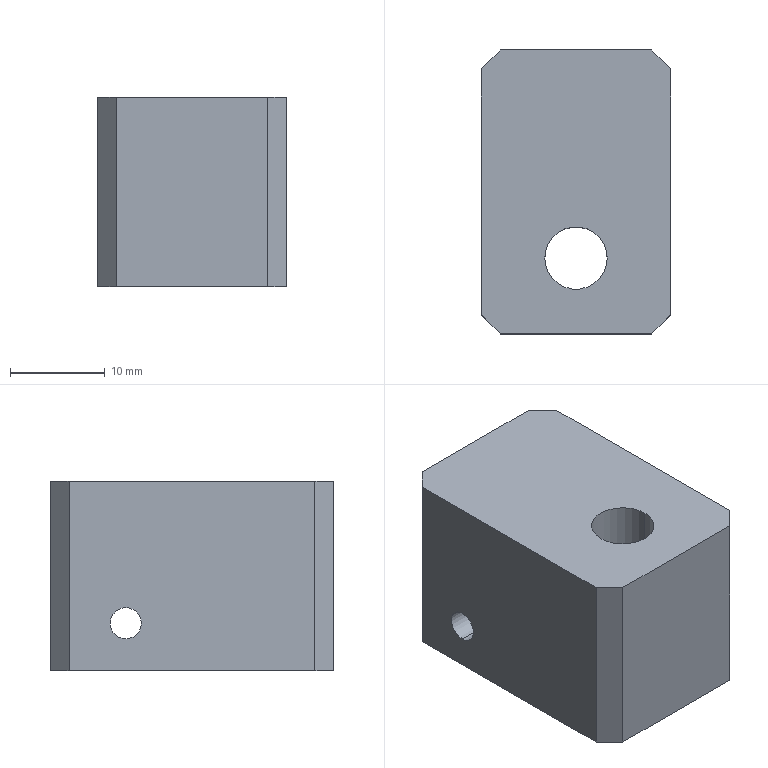Part | SolidWorks | features HoleWzd 2, Chamfer 1, Extrusion 1 | 1 solid | 17 faces | box 20 x 30 x 20 mm | volume 10571 mm3 | plane 11 | cylinder 6 | commonest cylinder face diameters 3.3 x2 6.6 x2 11 x2
STEP:
#1=CARTESIAN_POINT('',(10.,7.,3.35));
#2=VERTEX_POINT('',#1);
#3=CARTESIAN_POINT('',(10.,7.,6.65));
#4=VERTEX_POINT('',#3);
#5=CARTESIAN_POINT('',(10.,7.,5.));
#6=DIRECTION('',(-1.,0.,0.));
#7=DIRECTION('',(0.,0.,1.));
#8=AXIS2_PLACEMENT_3D('',#5,#6,#7);
#9=CIRCLE('',#8,1.65);
#10=EDGE_CURVE('',#2,#4,#9,.T.);
#11=ORIENTED_EDGE('',*,*,#10,.F.);
#12=CARTESIAN_POINT('',(-10.,7.,3.35));
#13=VERTEX_POINT('',#12);
#14=CARTESIAN_POINT('',(-10.,7.,3.35));
#15=DIRECTION('',(-1.,0.,0.));
#16=VECTOR('',#15,1000.);
#17=LINE('',#14,#16);
#18=EDGE_CURVE('',#2,#13,#17,.T.);
#19=ORIENTED_EDGE('',*,*,#18,.T.);
#20=CARTESIAN_POINT('',(-10.,7.,6.65));
#21=VERTEX_POINT('',#20);
#22=CARTESIAN_POINT('',(-10.,7.,5.));
#23=DIRECTION('',(-1.,0.,0.));
#24=DIRECTION('',(0.,0.,1.));
#25=AXIS2_PLACEMENT_3D('',#22,#23,#24);
#26=CIRCLE('',#25,1.65);
#27=EDGE_CURVE('',#13,#21,#26,.T.);
#28=ORIENTED_EDGE('',*,*,#27,.T.);
#29=CARTESIAN_POINT('',(-10.,7.,6.65));
#30=DIRECTION('',(-1.,0.,0.));
#31=VECTOR('',#30,1000.);
#32=LINE('',#29,#31);
#33=EDGE_CURVE('',#4,#21,#32,.T.);
#34=ORIENTED_EDGE('',*,*,#33,.F.);
#35=EDGE_LOOP('',(#11,#19,#28,#34));
#36=FACE_OUTER_BOUND('',#35,.T.);
#37=CARTESIAN_POINT('',(-10.,7.,5.));
#38=DIRECTION('',(-1.,0.,0.));
#39=DIRECTION('',(0.,0.,1.));
#40=AXIS2_PLACEMENT_3D('',#37,#38,#39);
#41=CYLINDRICAL_SURFACE('',#40,1.65);
#42=ADVANCED_FACE('',(#36),#41,.F.);
#43=CARTESIAN_POINT('',(5.5,-7.,6.8));
#44=VERTEX_POINT('',#43);
#45=CARTESIAN_POINT('',(-5.5,-7.,6.8));
#46=VERTEX_POINT('',#45);
#47=CARTESIAN_POINT('',(0.,-7.,6.8));
#48=DIRECTION('',(0.,0.,-1.));
#49=DIRECTION('',(-1.,0.,0.));
#50=AXIS2_PLACEMENT_3D('',#47,#48,#49);
#51=CIRCLE('',#50,5.5);
#52=EDGE_CURVE('',#44,#46,#51,.T.);
#53=ORIENTED_EDGE('',*,*,#52,.F.);
#54=CARTESIAN_POINT('',(5.5,-7.,0.));
#55=VERTEX_POINT('',#54);
#56=CARTESIAN_POINT('',(5.5,-7.,0.));
#57=DIRECTION('',(0.,0.,-1.));
#58=VECTOR('',#57,1000.);
#59=LINE('',#56,#58);
#60=EDGE_CURVE('',#44,#55,#59,.T.);
#61=ORIENTED_EDGE('',*,*,#60,.T.);
#62=CARTESIAN_POINT('',(-5.5,-7.,0.));
#63=VERTEX_POINT('',#62);
#64=CARTESIAN_POINT('',(0.,-7.,0.));
#65=DIRECTION('',(0.,0.,-1.));
#66=DIRECTION('',(-1.,0.,0.));
#67=AXIS2_PLACEMENT_3D('',#64,#65,#66);
#68=CIRCLE('',#67,5.5);
#69=EDGE_CURVE('',#55,#63,#68,.T.);
#70=ORIENTED_EDGE('',*,*,#69,.T.);
#71=CARTESIAN_POINT('',(-5.5,-7.,0.));
#72=DIRECTION('',(0.,0.,-1.));
#73=VECTOR('',#72,1000.);
#74=LINE('',#71,#73);
#75=EDGE_CURVE('',#46,#63,#74,.T.);
#76=ORIENTED_EDGE('',*,*,#75,.F.);
#77=EDGE_LOOP('',(#53,#61,#70,#76));
#78=FACE_OUTER_BOUND('',#77,.T.);
#79=CARTESIAN_POINT('',(0.,-7.,0.));
#80=DIRECTION('',(0.,0.,-1.));
#81=DIRECTION('',(-1.,0.,0.));
#82=AXIS2_PLACEMENT_3D('',#79,#80,#81);
#83=CYLINDRICAL_SURFACE('',#82,5.5);
#84=ADVANCED_FACE('',(#78),#83,.F.);
#85=CARTESIAN_POINT('',(3.3,-7.,20.));
#86=VERTEX_POINT('',#85);
#87=CARTESIAN_POINT('',(-3.3,-7.,20.));
#88=VERTEX_POINT('',#87);
#89=CARTESIAN_POINT('',(0.,-7.,20.));
#90=DIRECTION('',(0.,0.,-1.));
#91=DIRECTION('',(-1.,0.,0.));
#92=AXIS2_PLACEMENT_3D('',#89,#90,#91);
#93=CIRCLE('',#92,3.3);
#94=EDGE_CURVE('',#86,#88,#93,.T.);
#95=ORIENTED_EDGE('',*,*,#94,.F.);
#96=CARTESIAN_POINT('',(3.3,-7.,6.8));
#97=VERTEX_POINT('',#96);
#98=CARTESIAN_POINT('',(3.3,-7.,0.));
#99=DIRECTION('',(0.,0.,-1.));
#100=VECTOR('',#99,1000.);
#101=LINE('',#98,#100);
#102=EDGE_CURVE('',#86,#97,#101,.T.);
#103=ORIENTED_EDGE('',*,*,#102,.T.);
#104=CARTESIAN_POINT('',(-3.3,-7.,6.8));
#105=VERTEX_POINT('',#104);
#106=CARTESIAN_POINT('',(0.,-7.,6.8));
#107=DIRECTION('',(0.,0.,-1.));
#108=DIRECTION('',(-1.,0.,0.));
#109=AXIS2_PLACEMENT_3D('',#106,#107,#108);
#110=CIRCLE('',#109,3.3);
#111=EDGE_CURVE('',#97,#105,#110,.T.);
#112=ORIENTED_EDGE('',*,*,#111,.T.);
#113=CARTESIAN_POINT('',(-3.3,-7.,0.));
#114=DIRECTION('',(0.,0.,-1.));
#115=VECTOR('',#114,1000.);
#116=LINE('',#113,#115);
#117=EDGE_CURVE('',#88,#105,#116,.T.);
#118=ORIENTED_EDGE('',*,*,#117,.F.);
#119=EDGE_LOOP('',(#95,#103,#112,#118));
#120=FACE_OUTER_BOUND('',#119,.T.);
#121=CARTESIAN_POINT('',(0.,-7.,0.));
#122=DIRECTION('',(0.,0.,-1.));
#123=DIRECTION('',(-1.,0.,0.));
#124=AXIS2_PLACEMENT_3D('',#121,#122,#123);
#125=CYLINDRICAL_SURFACE('',#124,3.3);
#126=ADVANCED_FACE('',(#120),#125,.F.);
#127=CARTESIAN_POINT('',(10.,7.,5.));
#128=DIRECTION('',(-1.,0.,0.));
#129=DIRECTION('',(0.,0.,1.));
#130=AXIS2_PLACEMENT_3D('',#127,#128,#129);
#131=CIRCLE('',#130,1.65);
#132=EDGE_CURVE('',#4,#2,#131,.T.);
#133=ORIENTED_EDGE('',*,*,#132,.T.);
#134=ORIENTED_EDGE('',*,*,#10,.T.);
#135=EDGE_LOOP('',(#133,#134));
#136=FACE_BOUND('',#135,.T.);
#137=CARTESIAN_POINT('',(10.,-13.,0.));
#138=VERTEX_POINT('',#137);
#139=CARTESIAN_POINT('',(10.,13.,0.));
#140=VERTEX_POINT('',#139);
#141=CARTESIAN_POINT('',(10.,15.,0.));
#142=DIRECTION('',(0.,1.,0.));
#143=VECTOR('',#142,1000.);
#144=LINE('',#141,#143);
#145=EDGE_CURVE('',#138,#140,#144,.T.);
#146=ORIENTED_EDGE('',*,*,#145,.T.);
#147=CARTESIAN_POINT('',(10.,13.,20.));
#148=VERTEX_POINT('',#147);
#149=CARTESIAN_POINT('',(10.,13.,20.));
#150=DIRECTION('',(0.,0.,1.));
#151=VECTOR('',#150,1000.);
#152=LINE('',#149,#151);
#153=EDGE_CURVE('',#140,#148,#152,.T.);
#154=ORIENTED_EDGE('',*,*,#153,.T.);
#155=CARTESIAN_POINT('',(10.,-13.,20.));
#156=VERTEX_POINT('',#155);
#157=CARTESIAN_POINT('',(10.,15.,20.));
#158=DIRECTION('',(0.,1.,0.));
#159=VECTOR('',#158,1000.);
#160=LINE('',#157,#159);
#161=EDGE_CURVE('',#156,#148,#160,.T.);
#162=ORIENTED_EDGE('',*,*,#161,.F.);
#163=CARTESIAN_POINT('',(10.,-13.,20.));
#164=DIRECTION('',(0.,0.,-1.));
#165=VECTOR('',#164,1000.);
#166=LINE('',#163,#165);
#167=EDGE_CURVE('',#156,#138,#166,.T.);
#168=ORIENTED_EDGE('',*,*,#167,.T.);
#169=EDGE_LOOP('',(#146,#154,#162,#168));
#170=FACE_OUTER_BOUND('',#169,.T.);
#171=CARTESIAN_POINT('',(10.,15.,20.));
#172=DIRECTION('',(-1.,0.,0.));
#173=DIRECTION('',(0.,-1.,0.));
#174=AXIS2_PLACEMENT_3D('',#171,#172,#173);
#175=PLANE('',#174);
#176=ADVANCED_FACE('',(#136,#170),#175,.F.);
#177=CARTESIAN_POINT('',(8.,15.,0.));
#178=VERTEX_POINT('',#177);
#179=CARTESIAN_POINT('',(-8.,15.,0.));
#180=VERTEX_POINT('',#179);
#181=CARTESIAN_POINT('',(-10.,15.,0.));
#182=DIRECTION('',(-1.,0.,0.));
#183=VECTOR('',#182,1000.);
#184=LINE('',#181,#183);
#185=EDGE_CURVE('',#178,#180,#184,.T.);
#186=ORIENTED_EDGE('',*,*,#185,.T.);
#187=CARTESIAN_POINT('',(-8.,15.,20.));
#188=VERTEX_POINT('',#187);
#189=CARTESIAN_POINT('',(-8.,15.,20.));
#190=DIRECTION('',(0.,0.,1.));
#191=VECTOR('',#190,1000.);
#192=LINE('',#189,#191);
#193=EDGE_CURVE('',#180,#188,#192,.T.);
#194=ORIENTED_EDGE('',*,*,#193,.T.);
#195=CARTESIAN_POINT('',(8.,15.,20.));
#196=VERTEX_POINT('',#195);
#197=CARTESIAN_POINT('',(-10.,15.,20.));
#198=DIRECTION('',(-1.,0.,0.));
#199=VECTOR('',#198,1000.);
#200=LINE('',#197,#199);
#201=EDGE_CURVE('',#196,#188,#200,.T.);
#202=ORIENTED_EDGE('',*,*,#201,.F.);
#203=CARTESIAN_POINT('',(8.,15.,20.));
#204=DIRECTION('',(0.,0.,-1.));
#205=VECTOR('',#204,1000.);
#206=LINE('',#203,#205);
#207=EDGE_CURVE('',#196,#178,#206,.T.);
#208=ORIENTED_EDGE('',*,*,#207,.T.);
#209=EDGE_LOOP('',(#186,#194,#202,#208));
#210=FACE_OUTER_BOUND('',#209,.T.);
#211=CARTESIAN_POINT('',(-10.,15.,20.));
#212=DIRECTION('',(0.,-1.,0.));
#213=DIRECTION('',(0.,0.,-1.));
#214=AXIS2_PLACEMENT_3D('',#211,#212,#213);
#215=PLANE('',#214);
#216=ADVANCED_FACE('',(#210),#215,.F.);
#217=CARTESIAN_POINT('',(-10.,7.,5.));
#218=DIRECTION('',(-1.,0.,0.));
#219=DIRECTION('',(0.,0.,1.));
#220=AXIS2_PLACEMENT_3D('',#217,#218,#219);
#221=CIRCLE('',#220,1.65);
#222=EDGE_CURVE('',#21,#13,#221,.T.);
#223=ORIENTED_EDGE('',*,*,#222,.F.);
#224=ORIENTED_EDGE('',*,*,#27,.F.);
#225=EDGE_LOOP('',(#223,#224));
#226=FACE_BOUND('',#225,.T.);
#227=CARTESIAN_POINT('',(-10.,13.,0.));
#228=VERTEX_POINT('',#227);
#229=CARTESIAN_POINT('',(-10.,-13.,0.));
#230=VERTEX_POINT('',#229);
#231=CARTESIAN_POINT('',(-10.,15.,0.));
#232=DIRECTION('',(0.,-1.,0.));
#233=VECTOR('',#232,1000.);
#234=LINE('',#231,#233);
#235=EDGE_CURVE('',#228,#230,#234,.T.);
#236=ORIENTED_EDGE('',*,*,#235,.T.);
#237=CARTESIAN_POINT('',(-10.,-13.,20.));
#238=VERTEX_POINT('',#237);
#239=CARTESIAN_POINT('',(-10.,-13.,20.));
#240=DIRECTION('',(0.,0.,1.));
#241=VECTOR('',#240,1000.);
#242=LINE('',#239,#241);
#243=EDGE_CURVE('',#230,#238,#242,.T.);
#244=ORIENTED_EDGE('',*,*,#243,.T.);
#245=CARTESIAN_POINT('',(-10.,13.,20.));
#246=VERTEX_POINT('',#245);
#247=CARTESIAN_POINT('',(-10.,15.,20.));
#248=DIRECTION('',(0.,-1.,0.));
#249=VECTOR('',#248,1000.);
#250=LINE('',#247,#249);
#251=EDGE_CURVE('',#246,#238,#250,.T.);
#252=ORIENTED_EDGE('',*,*,#251,.F.);
#253=CARTESIAN_POINT('',(-10.,13.,20.));
#254=DIRECTION('',(0.,0.,-1.));
#255=VECTOR('',#254,1000.);
#256=LINE('',#253,#255);
#257=EDGE_CURVE('',#246,#228,#256,.T.);
#258=ORIENTED_EDGE('',*,*,#257,.T.);
#259=EDGE_LOOP('',(#236,#244,#252,#258));
#260=FACE_OUTER_BOUND('',#259,.T.);
#261=CARTESIAN_POINT('',(-10.,15.,20.));
#262=DIRECTION('',(1.,0.,0.));
#263=DIRECTION('',(0.,1.,0.));
#264=AXIS2_PLACEMENT_3D('',#261,#262,#263);
#265=PLANE('',#264);
#266=ADVANCED_FACE('',(#226,#260),#265,.F.);
#267=CARTESIAN_POINT('',(-8.,-15.,20.));
#268=VERTEX_POINT('',#267);
#269=CARTESIAN_POINT('',(8.,-15.,20.));
#270=VERTEX_POINT('',#269);
#271=CARTESIAN_POINT('',(-10.,-15.,20.));
#272=DIRECTION('',(1.,0.,0.));
#273=VECTOR('',#272,1000.);
#274=LINE('',#271,#273);
#275=EDGE_CURVE('',#268,#270,#274,.T.);
#276=ORIENTED_EDGE('',*,*,#275,.F.);
#277=CARTESIAN_POINT('',(-8.,-15.,0.));
#278=VERTEX_POINT('',#277);
#279=CARTESIAN_POINT('',(-8.,-15.,20.));
#280=DIRECTION('',(0.,0.,-1.));
#281=VECTOR('',#280,1000.);
#282=LINE('',#279,#281);
#283=EDGE_CURVE('',#268,#278,#282,.T.);
#284=ORIENTED_EDGE('',*,*,#283,.T.);
#285=CARTESIAN_POINT('',(8.,-15.,0.));
#286=VERTEX_POINT('',#285);
#287=CARTESIAN_POINT('',(-10.,-15.,0.));
#288=DIRECTION('',(1.,0.,0.));
#289=VECTOR('',#288,1000.);
#290=LINE('',#287,#289);
#291=EDGE_CURVE('',#278,#286,#290,.T.);
#292=ORIENTED_EDGE('',*,*,#291,.T.);
#293=CARTESIAN_POINT('',(8.,-15.,20.));
#294=DIRECTION('',(0.,0.,1.));
#295=VECTOR('',#294,1000.);
#296=LINE('',#293,#295);
#297=EDGE_CURVE('',#286,#270,#296,.T.);
#298=ORIENTED_EDGE('',*,*,#297,.T.);
#299=EDGE_LOOP('',(#276,#284,#292,#298));
#300=FACE_OUTER_BOUND('',#299,.T.);
#301=CARTESIAN_POINT('',(-10.,-15.,20.));
#302=DIRECTION('',(0.,1.,0.));
#303=DIRECTION('',(0.,0.,1.));
#304=AXIS2_PLACEMENT_3D('',#301,#302,#303);
#305=PLANE('',#304);
#306=ADVANCED_FACE('',(#300),#305,.F.);
#307=CARTESIAN_POINT('',(0.,-7.,20.));
#308=DIRECTION('',(0.,0.,-1.));
#309=DIRECTION('',(-1.,0.,0.));
#310=AXIS2_PLACEMENT_3D('',#307,#308,#309);
#311=CIRCLE('',#310,3.3);
#312=EDGE_CURVE('',#88,#86,#311,.T.);
#313=ORIENTED_EDGE('',*,*,#312,.T.);
#314=ORIENTED_EDGE('',*,*,#94,.T.);
#315=EDGE_LOOP('',(#313,#314));
#316=FACE_BOUND('',#315,.T.);
#317=ORIENTED_EDGE('',*,*,#251,.T.);
#318=CARTESIAN_POINT('',(1.,-24.,20.));
#319=DIRECTION('',(0.7071,-0.7071,0.));
#320=VECTOR('',#319,1000.);
#321=LINE('',#318,#320);
#322=EDGE_CURVE('',#238,#268,#321,.T.);
#323=ORIENTED_EDGE('',*,*,#322,.T.);
#324=ORIENTED_EDGE('',*,*,#275,.T.);
#325=CARTESIAN_POINT('',(9.,-14.,20.));
#326=DIRECTION('',(0.7071,0.7071,0.));
#327=VECTOR('',#326,1000.);
#328=LINE('',#325,#327);
#329=EDGE_CURVE('',#270,#156,#328,.T.);
#330=ORIENTED_EDGE('',*,*,#329,.T.);
#331=ORIENTED_EDGE('',*,*,#161,.T.);
#332=CARTESIAN_POINT('',(24.,-1.,20.));
#333=DIRECTION('',(-0.7071,0.7071,0.));
#334=VECTOR('',#333,1000.);
#335=LINE('',#332,#334);
#336=EDGE_CURVE('',#148,#196,#335,.T.);
#337=ORIENTED_EDGE('',*,*,#336,.T.);
#338=ORIENTED_EDGE('',*,*,#201,.T.);
#339=CARTESIAN_POINT('',(-14.,9.,20.));
#340=DIRECTION('',(-0.7071,-0.7071,0.));
#341=VECTOR('',#340,1000.);
#342=LINE('',#339,#341);
#343=EDGE_CURVE('',#188,#246,#342,.T.);
#344=ORIENTED_EDGE('',*,*,#343,.T.);
#345=EDGE_LOOP('',(#317,#323,#324,#330,#331,#337,#338,#344));
#346=FACE_OUTER_BOUND('',#345,.T.);
#347=CARTESIAN_POINT('',(10.,-15.,20.));
#348=DIRECTION('',(0.,0.,1.));
#349=DIRECTION('',(1.,0.,0.));
#350=AXIS2_PLACEMENT_3D('',#347,#348,#349);
#351=PLANE('',#350);
#352=ADVANCED_FACE('',(#316,#346),#351,.T.);
#353=CARTESIAN_POINT('',(0.,-7.,0.));
#354=DIRECTION('',(0.,0.,-1.));
#355=DIRECTION('',(-1.,0.,0.));
#356=AXIS2_PLACEMENT_3D('',#353,#354,#355);
#357=CIRCLE('',#356,5.5);
#358=EDGE_CURVE('',#63,#55,#357,.T.);
#359=ORIENTED_EDGE('',*,*,#358,.F.);
#360=ORIENTED_EDGE('',*,*,#69,.F.);
#361=EDGE_LOOP('',(#359,#360));
#362=FACE_BOUND('',#361,.T.);
#363=ORIENTED_EDGE('',*,*,#291,.F.);
#364=CARTESIAN_POINT('',(-8.,-15.,0.));
#365=DIRECTION('',(-0.7071,0.7071,0.));
#366=VECTOR('',#365,1000.);
#367=LINE('',#364,#366);
#368=EDGE_CURVE('',#278,#230,#367,.T.);
#369=ORIENTED_EDGE('',*,*,#368,.T.);
#370=ORIENTED_EDGE('',*,*,#235,.F.);
#371=CARTESIAN_POINT('',(-10.,13.,0.));
#372=DIRECTION('',(0.7071,0.7071,0.));
#373=VECTOR('',#372,1000.);
#374=LINE('',#371,#373);
#375=EDGE_CURVE('',#228,#180,#374,.T.);
#376=ORIENTED_EDGE('',*,*,#375,.T.);
#377=ORIENTED_EDGE('',*,*,#185,.F.);
#378=CARTESIAN_POINT('',(8.,15.,0.));
#379=DIRECTION('',(0.7071,-0.7071,0.));
#380=VECTOR('',#379,1000.);
#381=LINE('',#378,#380);
#382=EDGE_CURVE('',#178,#140,#381,.T.);
#383=ORIENTED_EDGE('',*,*,#382,.T.);
#384=ORIENTED_EDGE('',*,*,#145,.F.);
#385=CARTESIAN_POINT('',(10.,-13.,0.));
#386=DIRECTION('',(-0.7071,-0.7071,0.));
#387=VECTOR('',#386,1000.);
#388=LINE('',#385,#387);
#389=EDGE_CURVE('',#138,#286,#388,.T.);
#390=ORIENTED_EDGE('',*,*,#389,.T.);
#391=EDGE_LOOP('',(#363,#369,#370,#376,#377,#383,#384,#390));
#392=FACE_OUTER_BOUND('',#391,.T.);
#393=CARTESIAN_POINT('',(10.,-15.,0.));
#394=DIRECTION('',(0.,0.,1.));
#395=DIRECTION('',(1.,0.,0.));
#396=AXIS2_PLACEMENT_3D('',#393,#394,#395);
#397=PLANE('',#396);
#398=ADVANCED_FACE('',(#362,#392),#397,.F.);
#399=ORIENTED_EDGE('',*,*,#102,.F.);
#400=ORIENTED_EDGE('',*,*,#312,.F.);
#401=ORIENTED_EDGE('',*,*,#117,.T.);
#402=CARTESIAN_POINT('',(0.,-7.,6.8));
#403=DIRECTION('',(0.,0.,-1.));
#404=DIRECTION('',(-1.,0.,0.));
#405=AXIS2_PLACEMENT_3D('',#402,#403,#404);
#406=CIRCLE('',#405,3.3);
#407=EDGE_CURVE('',#105,#97,#406,.T.);
#408=ORIENTED_EDGE('',*,*,#407,.T.);
#409=EDGE_LOOP('',(#399,#400,#401,#408));
#410=FACE_OUTER_BOUND('',#409,.T.);
#411=CARTESIAN_POINT('',(0.,-7.,0.));
#412=DIRECTION('',(0.,0.,-1.));
#413=DIRECTION('',(-1.,0.,0.));
#414=AXIS2_PLACEMENT_3D('',#411,#412,#413);
#415=CYLINDRICAL_SURFACE('',#414,3.3);
#416=ADVANCED_FACE('',(#410),#415,.F.);
#417=ORIENTED_EDGE('',*,*,#407,.F.);
#418=ORIENTED_EDGE('',*,*,#111,.F.);
#419=EDGE_LOOP('',(#417,#418));
#420=FACE_BOUND('',#419,.T.);
#421=CARTESIAN_POINT('',(0.,-7.,6.8));
#422=DIRECTION('',(0.,0.,-1.));
#423=DIRECTION('',(-1.,0.,0.));
#424=AXIS2_PLACEMENT_3D('',#421,#422,#423);
#425=CIRCLE('',#424,5.5);
#426=EDGE_CURVE('',#46,#44,#425,.T.);
#427=ORIENTED_EDGE('',*,*,#426,.T.);
#428=ORIENTED_EDGE('',*,*,#52,.T.);
#429=EDGE_LOOP('',(#427,#428));
#430=FACE_OUTER_BOUND('',#429,.T.);
#431=CARTESIAN_POINT('',(3.3,-7.,6.8));
#432=DIRECTION('',(0.,0.,1.));
#433=DIRECTION('',(1.,0.,0.));
#434=AXIS2_PLACEMENT_3D('',#431,#432,#433);
#435=PLANE('',#434);
#436=ADVANCED_FACE('',(#420,#430),#435,.F.);
#437=ORIENTED_EDGE('',*,*,#60,.F.);
#438=ORIENTED_EDGE('',*,*,#426,.F.);
#439=ORIENTED_EDGE('',*,*,#75,.T.);
#440=ORIENTED_EDGE('',*,*,#358,.T.);
#441=EDGE_LOOP('',(#437,#438,#439,#440));
#442=FACE_OUTER_BOUND('',#441,.T.);
#443=CARTESIAN_POINT('',(0.,-7.,0.));
#444=DIRECTION('',(0.,0.,-1.));
#445=DIRECTION('',(-1.,0.,0.));
#446=AXIS2_PLACEMENT_3D('',#443,#444,#445);
#447=CYLINDRICAL_SURFACE('',#446,5.5);
#448=ADVANCED_FACE('',(#442),#447,.F.);
#449=ORIENTED_EDGE('',*,*,#18,.F.);
#450=ORIENTED_EDGE('',*,*,#132,.F.);
#451=ORIENTED_EDGE('',*,*,#33,.T.);
#452=ORIENTED_EDGE('',*,*,#222,.T.);
#453=EDGE_LOOP('',(#449,#450,#451,#452));
#454=FACE_OUTER_BOUND('',#453,.T.);
#455=CARTESIAN_POINT('',(-10.,7.,5.));
#456=DIRECTION('',(-1.,0.,0.));
#457=DIRECTION('',(0.,0.,1.));
#458=AXIS2_PLACEMENT_3D('',#455,#456,#457);
#459=CYLINDRICAL_SURFACE('',#458,1.65);
#460=ADVANCED_FACE('',(#454),#459,.F.);
#461=ORIENTED_EDGE('',*,*,#322,.F.);
#462=ORIENTED_EDGE('',*,*,#243,.F.);
#463=ORIENTED_EDGE('',*,*,#368,.F.);
#464=ORIENTED_EDGE('',*,*,#283,.F.);
#465=EDGE_LOOP('',(#461,#462,#463,#464));
#466=FACE_OUTER_BOUND('',#465,.T.);
#467=CARTESIAN_POINT('',(-8.,-15.,20.));
#468=DIRECTION('',(0.7071,0.7071,0.));
#469=DIRECTION('',(0.,0.,-1.));
#470=AXIS2_PLACEMENT_3D('',#467,#468,#469);
#471=PLANE('',#470);
#472=ADVANCED_FACE('',(#466),#471,.F.);
#473=ORIENTED_EDGE('',*,*,#343,.F.);
#474=ORIENTED_EDGE('',*,*,#193,.F.);
#475=ORIENTED_EDGE('',*,*,#375,.F.);
#476=ORIENTED_EDGE('',*,*,#257,.F.);
#477=EDGE_LOOP('',(#473,#474,#475,#476));
#478=FACE_OUTER_BOUND('',#477,.T.);
#479=CARTESIAN_POINT('',(-10.,13.,20.));
#480=DIRECTION('',(0.7071,-0.7071,0.));
#481=DIRECTION('',(0.,0.,-1.));
#482=AXIS2_PLACEMENT_3D('',#479,#480,#481);
#483=PLANE('',#482);
#484=ADVANCED_FACE('',(#478),#483,.F.);
#485=ORIENTED_EDGE('',*,*,#336,.F.);
#486=ORIENTED_EDGE('',*,*,#153,.F.);
#487=ORIENTED_EDGE('',*,*,#382,.F.);
#488=ORIENTED_EDGE('',*,*,#207,.F.);
#489=EDGE_LOOP('',(#485,#486,#487,#488));
#490=FACE_OUTER_BOUND('',#489,.T.);
#491=CARTESIAN_POINT('',(8.,15.,20.));
#492=DIRECTION('',(-0.7071,-0.7071,0.));
#493=DIRECTION('',(0.,0.,-1.));
#494=AXIS2_PLACEMENT_3D('',#491,#492,#493);
#495=PLANE('',#494);
#496=ADVANCED_FACE('',(#490),#495,.F.);
#497=ORIENTED_EDGE('',*,*,#329,.F.);
#498=ORIENTED_EDGE('',*,*,#297,.F.);
#499=ORIENTED_EDGE('',*,*,#389,.F.);
#500=ORIENTED_EDGE('',*,*,#167,.F.);
#501=EDGE_LOOP('',(#497,#498,#499,#500));
#502=FACE_OUTER_BOUND('',#501,.T.);
#503=CARTESIAN_POINT('',(10.,-13.,20.));
#504=DIRECTION('',(-0.7071,0.7071,0.));
#505=DIRECTION('',(0.,0.,-1.));
#506=AXIS2_PLACEMENT_3D('',#503,#504,#505);
#507=PLANE('',#506);
#508=ADVANCED_FACE('',(#502),#507,.F.);
#509=CLOSED_SHELL('',(#42,#84,#126,#176,#216,#266,#306,#352,#398,#416,#436,#448,#460,#472,#484,#496,#508));
#510=MANIFOLD_SOLID_BREP('',#509);
#511=CARTESIAN_POINT('',(0.,0.,0.));
#512=DIRECTION('',(0.,0.,1.));
#513=DIRECTION('',(1.,0.,0.));
#514=AXIS2_PLACEMENT_3D('',#511,#512,#513);
#515=(LENGTH_UNIT()NAMED_UNIT(*)SI_UNIT(.MILLI.,.METRE.));
#516=UNCERTAINTY_MEASURE_WITH_UNIT(LENGTH_MEASURE(0.00001),#515,'','');
#517=(NAMED_UNIT(*)PLANE_ANGLE_UNIT()SI_UNIT($,.RADIAN.));
#518=(NAMED_UNIT(*)SI_UNIT($,.STERADIAN.)SOLID_ANGLE_UNIT());
#519=(GEOMETRIC_REPRESENTATION_CONTEXT(3)GLOBAL_UNCERTAINTY_ASSIGNED_CONTEXT((#516))GLOBAL_UNIT_ASSIGNED_CONTEXT((#515,#517,#518))REPRESENTATION_CONTEXT('',''));
#520=ADVANCED_BREP_SHAPE_REPRESENTATION('',(#510,#514),#519);